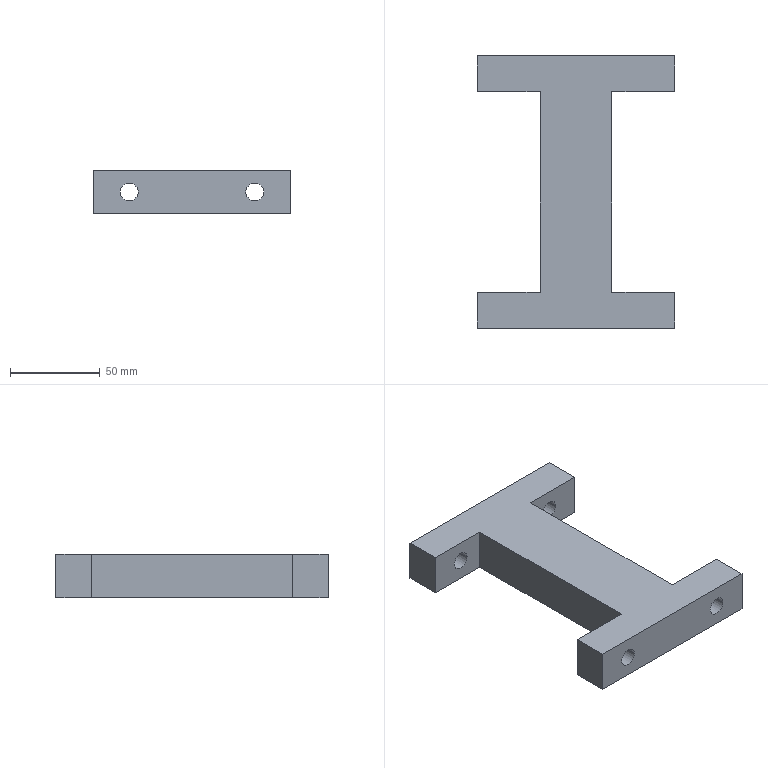Part | SolidWorks | features BaseBody 1 | 1 solid | 22 faces | box 110 x 152 x 24 mm | volume 206837 mm3 | plane 14 | cylinder 8 | commonest cylinder face diameters 10 x8
STEP:
#1=CARTESIAN_POINT('',(30.,-20.,0.));
#2=VERTEX_POINT('',#1);
#3=CARTESIAN_POINT('',(40.,-20.,0.));
#4=VERTEX_POINT('',#3);
#5=CARTESIAN_POINT('',(35.,-20.,0.));
#6=DIRECTION('',(0.,-1.,0.));
#7=DIRECTION('',(-1.,0.,0.));
#8=AXIS2_PLACEMENT_3D('',#5,#6,#7);
#9=CIRCLE('',#8,5.);
#10=EDGE_CURVE('',#2,#4,#9,.T.);
#11=ORIENTED_EDGE('',*,*,#10,.T.);
#12=CARTESIAN_POINT('',(40.,0.,0.));
#13=VERTEX_POINT('',#12);
#14=CARTESIAN_POINT('',(40.,-152.,0.));
#15=DIRECTION('',(0.,1.,0.));
#16=VECTOR('',#15,1000.);
#17=LINE('',#14,#16);
#18=EDGE_CURVE('',#4,#13,#17,.T.);
#19=ORIENTED_EDGE('',*,*,#18,.T.);
#20=CARTESIAN_POINT('',(30.,0.,0.));
#21=VERTEX_POINT('',#20);
#22=CARTESIAN_POINT('',(35.,0.,0.));
#23=DIRECTION('',(0.,1.,0.));
#24=DIRECTION('',(-1.,0.,0.));
#25=AXIS2_PLACEMENT_3D('',#22,#23,#24);
#26=CIRCLE('',#25,5.);
#27=EDGE_CURVE('',#13,#21,#26,.T.);
#28=ORIENTED_EDGE('',*,*,#27,.T.);
#29=CARTESIAN_POINT('',(30.,-152.,0.));
#30=DIRECTION('',(0.,1.,0.));
#31=VECTOR('',#30,1000.);
#32=LINE('',#29,#31);
#33=EDGE_CURVE('',#2,#21,#32,.T.);
#34=ORIENTED_EDGE('',*,*,#33,.F.);
#35=EDGE_LOOP('',(#11,#19,#28,#34));
#36=FACE_OUTER_BOUND('',#35,.T.);
#37=CARTESIAN_POINT('',(35.,-152.,0.));
#38=DIRECTION('',(0.,1.,0.));
#39=DIRECTION('',(-1.,0.,0.));
#40=AXIS2_PLACEMENT_3D('',#37,#38,#39);
#41=CYLINDRICAL_SURFACE('',#40,5.);
#42=ADVANCED_FACE('',(#36),#41,.F.);
#43=CARTESIAN_POINT('',(-40.,-20.,0.));
#44=VERTEX_POINT('',#43);
#45=CARTESIAN_POINT('',(-30.,-20.,0.));
#46=VERTEX_POINT('',#45);
#47=CARTESIAN_POINT('',(-35.,-20.,0.));
#48=DIRECTION('',(0.,-1.,0.));
#49=DIRECTION('',(-1.,0.,0.));
#50=AXIS2_PLACEMENT_3D('',#47,#48,#49);
#51=CIRCLE('',#50,5.);
#52=EDGE_CURVE('',#44,#46,#51,.T.);
#53=ORIENTED_EDGE('',*,*,#52,.T.);
#54=CARTESIAN_POINT('',(-30.,0.,0.));
#55=VERTEX_POINT('',#54);
#56=CARTESIAN_POINT('',(-30.,-152.,0.));
#57=DIRECTION('',(0.,1.,0.));
#58=VECTOR('',#57,1000.);
#59=LINE('',#56,#58);
#60=EDGE_CURVE('',#46,#55,#59,.T.);
#61=ORIENTED_EDGE('',*,*,#60,.T.);
#62=CARTESIAN_POINT('',(-40.,0.,0.));
#63=VERTEX_POINT('',#62);
#64=CARTESIAN_POINT('',(-35.,0.,0.));
#65=DIRECTION('',(0.,1.,0.));
#66=DIRECTION('',(-1.,0.,0.));
#67=AXIS2_PLACEMENT_3D('',#64,#65,#66);
#68=CIRCLE('',#67,5.);
#69=EDGE_CURVE('',#55,#63,#68,.T.);
#70=ORIENTED_EDGE('',*,*,#69,.T.);
#71=CARTESIAN_POINT('',(-40.,-152.,0.));
#72=DIRECTION('',(0.,1.,0.));
#73=VECTOR('',#72,1000.);
#74=LINE('',#71,#73);
#75=EDGE_CURVE('',#44,#63,#74,.T.);
#76=ORIENTED_EDGE('',*,*,#75,.F.);
#77=EDGE_LOOP('',(#53,#61,#70,#76));
#78=FACE_OUTER_BOUND('',#77,.T.);
#79=CARTESIAN_POINT('',(-35.,-152.,0.));
#80=DIRECTION('',(0.,1.,0.));
#81=DIRECTION('',(-1.,0.,0.));
#82=AXIS2_PLACEMENT_3D('',#79,#80,#81);
#83=CYLINDRICAL_SURFACE('',#82,5.);
#84=ADVANCED_FACE('',(#78),#83,.F.);
#85=CARTESIAN_POINT('',(30.,-152.,0.));
#86=VERTEX_POINT('',#85);
#87=CARTESIAN_POINT('',(40.,-152.,0.));
#88=VERTEX_POINT('',#87);
#89=CARTESIAN_POINT('',(35.,-152.,0.));
#90=DIRECTION('',(0.,-1.,0.));
#91=DIRECTION('',(-1.,0.,0.));
#92=AXIS2_PLACEMENT_3D('',#89,#90,#91);
#93=CIRCLE('',#92,5.);
#94=EDGE_CURVE('',#86,#88,#93,.T.);
#95=ORIENTED_EDGE('',*,*,#94,.T.);
#96=CARTESIAN_POINT('',(40.,-132.,0.));
#97=VERTEX_POINT('',#96);
#98=CARTESIAN_POINT('',(40.,-152.,0.));
#99=DIRECTION('',(0.,1.,0.));
#100=VECTOR('',#99,1000.);
#101=LINE('',#98,#100);
#102=EDGE_CURVE('',#88,#97,#101,.T.);
#103=ORIENTED_EDGE('',*,*,#102,.T.);
#104=CARTESIAN_POINT('',(30.,-132.,0.));
#105=VERTEX_POINT('',#104);
#106=CARTESIAN_POINT('',(35.,-132.,0.));
#107=DIRECTION('',(0.,1.,0.));
#108=DIRECTION('',(-1.,0.,0.));
#109=AXIS2_PLACEMENT_3D('',#106,#107,#108);
#110=CIRCLE('',#109,5.);
#111=EDGE_CURVE('',#97,#105,#110,.T.);
#112=ORIENTED_EDGE('',*,*,#111,.T.);
#113=CARTESIAN_POINT('',(30.,-152.,0.));
#114=DIRECTION('',(0.,1.,0.));
#115=VECTOR('',#114,1000.);
#116=LINE('',#113,#115);
#117=EDGE_CURVE('',#86,#105,#116,.T.);
#118=ORIENTED_EDGE('',*,*,#117,.F.);
#119=EDGE_LOOP('',(#95,#103,#112,#118));
#120=FACE_OUTER_BOUND('',#119,.T.);
#121=CARTESIAN_POINT('',(35.,-152.,0.));
#122=DIRECTION('',(0.,1.,0.));
#123=DIRECTION('',(-1.,0.,0.));
#124=AXIS2_PLACEMENT_3D('',#121,#122,#123);
#125=CYLINDRICAL_SURFACE('',#124,5.);
#126=ADVANCED_FACE('',(#120),#125,.F.);
#127=CARTESIAN_POINT('',(-40.,-152.,0.));
#128=VERTEX_POINT('',#127);
#129=CARTESIAN_POINT('',(-30.,-152.,0.));
#130=VERTEX_POINT('',#129);
#131=CARTESIAN_POINT('',(-35.,-152.,0.));
#132=DIRECTION('',(0.,-1.,0.));
#133=DIRECTION('',(-1.,0.,0.));
#134=AXIS2_PLACEMENT_3D('',#131,#132,#133);
#135=CIRCLE('',#134,5.);
#136=EDGE_CURVE('',#128,#130,#135,.T.);
#137=ORIENTED_EDGE('',*,*,#136,.T.);
#138=CARTESIAN_POINT('',(-30.,-132.,0.));
#139=VERTEX_POINT('',#138);
#140=CARTESIAN_POINT('',(-30.,-152.,0.));
#141=DIRECTION('',(0.,1.,0.));
#142=VECTOR('',#141,1000.);
#143=LINE('',#140,#142);
#144=EDGE_CURVE('',#130,#139,#143,.T.);
#145=ORIENTED_EDGE('',*,*,#144,.T.);
#146=CARTESIAN_POINT('',(-40.,-132.,0.));
#147=VERTEX_POINT('',#146);
#148=CARTESIAN_POINT('',(-35.,-132.,0.));
#149=DIRECTION('',(0.,1.,0.));
#150=DIRECTION('',(-1.,0.,0.));
#151=AXIS2_PLACEMENT_3D('',#148,#149,#150);
#152=CIRCLE('',#151,5.);
#153=EDGE_CURVE('',#139,#147,#152,.T.);
#154=ORIENTED_EDGE('',*,*,#153,.T.);
#155=CARTESIAN_POINT('',(-40.,-152.,0.));
#156=DIRECTION('',(0.,1.,0.));
#157=VECTOR('',#156,1000.);
#158=LINE('',#155,#157);
#159=EDGE_CURVE('',#128,#147,#158,.T.);
#160=ORIENTED_EDGE('',*,*,#159,.F.);
#161=EDGE_LOOP('',(#137,#145,#154,#160));
#162=FACE_OUTER_BOUND('',#161,.T.);
#163=CARTESIAN_POINT('',(-35.,-152.,0.));
#164=DIRECTION('',(0.,1.,0.));
#165=DIRECTION('',(-1.,0.,0.));
#166=AXIS2_PLACEMENT_3D('',#163,#164,#165);
#167=CYLINDRICAL_SURFACE('',#166,5.);
#168=ADVANCED_FACE('',(#162),#167,.F.);
#169=CARTESIAN_POINT('',(55.,-20.,12.));
#170=VERTEX_POINT('',#169);
#171=CARTESIAN_POINT('',(55.,0.,12.));
#172=VERTEX_POINT('',#171);
#173=CARTESIAN_POINT('',(55.,0.,12.));
#174=DIRECTION('',(0.,1.,0.));
#175=VECTOR('',#174,1000.);
#176=LINE('',#173,#175);
#177=EDGE_CURVE('',#170,#172,#176,.T.);
#178=ORIENTED_EDGE('',*,*,#177,.T.);
#179=CARTESIAN_POINT('',(-55.,0.,12.));
#180=VERTEX_POINT('',#179);
#181=CARTESIAN_POINT('',(0.,0.,12.));
#182=DIRECTION('',(-1.,0.,0.));
#183=VECTOR('',#182,1000.);
#184=LINE('',#181,#183);
#185=EDGE_CURVE('',#172,#180,#184,.T.);
#186=ORIENTED_EDGE('',*,*,#185,.T.);
#187=CARTESIAN_POINT('',(-55.,-20.,12.));
#188=VERTEX_POINT('',#187);
#189=CARTESIAN_POINT('',(-55.,0.,12.));
#190=DIRECTION('',(0.,-1.,0.));
#191=VECTOR('',#190,1000.);
#192=LINE('',#189,#191);
#193=EDGE_CURVE('',#180,#188,#192,.T.);
#194=ORIENTED_EDGE('',*,*,#193,.T.);
#195=CARTESIAN_POINT('',(-20.,-20.,12.));
#196=VERTEX_POINT('',#195);
#197=CARTESIAN_POINT('',(0.,-20.,12.));
#198=DIRECTION('',(1.,0.,0.));
#199=VECTOR('',#198,1000.);
#200=LINE('',#197,#199);
#201=EDGE_CURVE('',#188,#196,#200,.T.);
#202=ORIENTED_EDGE('',*,*,#201,.T.);
#203=CARTESIAN_POINT('',(-20.,-132.,12.));
#204=VERTEX_POINT('',#203);
#205=CARTESIAN_POINT('',(-20.,0.,12.));
#206=DIRECTION('',(0.,-1.,0.));
#207=VECTOR('',#206,1000.);
#208=LINE('',#205,#207);
#209=EDGE_CURVE('',#196,#204,#208,.T.);
#210=ORIENTED_EDGE('',*,*,#209,.T.);
#211=CARTESIAN_POINT('',(-55.,-132.,12.));
#212=VERTEX_POINT('',#211);
#213=CARTESIAN_POINT('',(0.,-132.,12.));
#214=DIRECTION('',(-1.,0.,0.));
#215=VECTOR('',#214,1000.);
#216=LINE('',#213,#215);
#217=EDGE_CURVE('',#204,#212,#216,.T.);
#218=ORIENTED_EDGE('',*,*,#217,.T.);
#219=CARTESIAN_POINT('',(-55.,-152.,12.));
#220=VERTEX_POINT('',#219);
#221=CARTESIAN_POINT('',(-55.,0.,12.));
#222=DIRECTION('',(0.,-1.,0.));
#223=VECTOR('',#222,1000.);
#224=LINE('',#221,#223);
#225=EDGE_CURVE('',#212,#220,#224,.T.);
#226=ORIENTED_EDGE('',*,*,#225,.T.);
#227=CARTESIAN_POINT('',(55.,-152.,12.));
#228=VERTEX_POINT('',#227);
#229=CARTESIAN_POINT('',(0.,-152.,12.));
#230=DIRECTION('',(1.,0.,0.));
#231=VECTOR('',#230,1000.);
#232=LINE('',#229,#231);
#233=EDGE_CURVE('',#220,#228,#232,.T.);
#234=ORIENTED_EDGE('',*,*,#233,.T.);
#235=CARTESIAN_POINT('',(55.,-132.,12.));
#236=VERTEX_POINT('',#235);
#237=CARTESIAN_POINT('',(55.,0.,12.));
#238=DIRECTION('',(0.,1.,0.));
#239=VECTOR('',#238,1000.);
#240=LINE('',#237,#239);
#241=EDGE_CURVE('',#228,#236,#240,.T.);
#242=ORIENTED_EDGE('',*,*,#241,.T.);
#243=CARTESIAN_POINT('',(20.,-132.,12.));
#244=VERTEX_POINT('',#243);
#245=CARTESIAN_POINT('',(0.,-132.,12.));
#246=DIRECTION('',(-1.,0.,0.));
#247=VECTOR('',#246,1000.);
#248=LINE('',#245,#247);
#249=EDGE_CURVE('',#236,#244,#248,.T.);
#250=ORIENTED_EDGE('',*,*,#249,.T.);
#251=CARTESIAN_POINT('',(20.,-20.,12.));
#252=VERTEX_POINT('',#251);
#253=CARTESIAN_POINT('',(20.,0.,12.));
#254=DIRECTION('',(0.,1.,0.));
#255=VECTOR('',#254,1000.);
#256=LINE('',#253,#255);
#257=EDGE_CURVE('',#244,#252,#256,.T.);
#258=ORIENTED_EDGE('',*,*,#257,.T.);
#259=CARTESIAN_POINT('',(0.,-20.,12.));
#260=DIRECTION('',(1.,0.,0.));
#261=VECTOR('',#260,1000.);
#262=LINE('',#259,#261);
#263=EDGE_CURVE('',#252,#170,#262,.T.);
#264=ORIENTED_EDGE('',*,*,#263,.T.);
#265=EDGE_LOOP('',(#178,#186,#194,#202,#210,#218,#226,#234,#242,#250,#258,#264));
#266=FACE_OUTER_BOUND('',#265,.T.);
#267=CARTESIAN_POINT('',(0.,0.,12.));
#268=DIRECTION('',(0.,0.,1.));
#269=DIRECTION('',(1.,0.,0.));
#270=AXIS2_PLACEMENT_3D('',#267,#268,#269);
#271=PLANE('',#270);
#272=ADVANCED_FACE('',(#266),#271,.T.);
#273=CARTESIAN_POINT('',(-55.,0.,-12.));
#274=VERTEX_POINT('',#273);
#275=CARTESIAN_POINT('',(-55.,0.,12.));
#276=DIRECTION('',(0.,0.,-1.));
#277=VECTOR('',#276,1000.);
#278=LINE('',#275,#277);
#279=EDGE_CURVE('',#180,#274,#278,.T.);
#280=ORIENTED_EDGE('',*,*,#279,.F.);
#281=ORIENTED_EDGE('',*,*,#185,.F.);
#282=CARTESIAN_POINT('',(55.,0.,-12.));
#283=VERTEX_POINT('',#282);
#284=CARTESIAN_POINT('',(55.,0.,12.));
#285=DIRECTION('',(0.,0.,1.));
#286=VECTOR('',#285,1000.);
#287=LINE('',#284,#286);
#288=EDGE_CURVE('',#283,#172,#287,.T.);
#289=ORIENTED_EDGE('',*,*,#288,.F.);
#290=CARTESIAN_POINT('',(-55.,0.,-12.));
#291=DIRECTION('',(1.,0.,0.));
#292=VECTOR('',#291,1000.);
#293=LINE('',#290,#292);
#294=EDGE_CURVE('',#274,#283,#293,.T.);
#295=ORIENTED_EDGE('',*,*,#294,.F.);
#296=EDGE_LOOP('',(#280,#281,#289,#295));
#297=FACE_OUTER_BOUND('',#296,.T.);
#298=CARTESIAN_POINT('',(35.,0.,0.));
#299=DIRECTION('',(0.,1.,0.));
#300=DIRECTION('',(-1.,0.,0.));
#301=AXIS2_PLACEMENT_3D('',#298,#299,#300);
#302=CIRCLE('',#301,5.);
#303=EDGE_CURVE('',#21,#13,#302,.T.);
#304=ORIENTED_EDGE('',*,*,#303,.F.);
#305=ORIENTED_EDGE('',*,*,#27,.F.);
#306=EDGE_LOOP('',(#304,#305));
#307=FACE_BOUND('',#306,.T.);
#308=CARTESIAN_POINT('',(-35.,0.,0.));
#309=DIRECTION('',(0.,1.,0.));
#310=DIRECTION('',(-1.,0.,0.));
#311=AXIS2_PLACEMENT_3D('',#308,#309,#310);
#312=CIRCLE('',#311,5.);
#313=EDGE_CURVE('',#63,#55,#312,.T.);
#314=ORIENTED_EDGE('',*,*,#313,.F.);
#315=ORIENTED_EDGE('',*,*,#69,.F.);
#316=EDGE_LOOP('',(#314,#315));
#317=FACE_BOUND('',#316,.T.);
#318=CARTESIAN_POINT('',(-55.,0.,12.));
#319=DIRECTION('',(0.,-1.,0.));
#320=DIRECTION('',(1.,0.,0.));
#321=AXIS2_PLACEMENT_3D('',#318,#319,#320);
#322=PLANE('',#321);
#323=ADVANCED_FACE('',(#297,#307,#317),#322,.F.);
#324=ORIENTED_EDGE('',*,*,#288,.T.);
#325=ORIENTED_EDGE('',*,*,#177,.F.);
#326=CARTESIAN_POINT('',(55.,-20.,-12.));
#327=VERTEX_POINT('',#326);
#328=CARTESIAN_POINT('',(55.,-20.,12.));
#329=DIRECTION('',(0.,0.,1.));
#330=VECTOR('',#329,1000.);
#331=LINE('',#328,#330);
#332=EDGE_CURVE('',#327,#170,#331,.T.);
#333=ORIENTED_EDGE('',*,*,#332,.F.);
#334=CARTESIAN_POINT('',(55.,0.,-12.));
#335=DIRECTION('',(0.,-1.,0.));
#336=VECTOR('',#335,1000.);
#337=LINE('',#334,#336);
#338=EDGE_CURVE('',#283,#327,#337,.T.);
#339=ORIENTED_EDGE('',*,*,#338,.F.);
#340=EDGE_LOOP('',(#324,#325,#333,#339));
#341=FACE_OUTER_BOUND('',#340,.T.);
#342=CARTESIAN_POINT('',(55.,0.,12.));
#343=DIRECTION('',(-1.,0.,0.));
#344=DIRECTION('',(0.,0.,1.));
#345=AXIS2_PLACEMENT_3D('',#342,#343,#344);
#346=PLANE('',#345);
#347=ADVANCED_FACE('',(#341),#346,.F.);
#348=ORIENTED_EDGE('',*,*,#332,.T.);
#349=ORIENTED_EDGE('',*,*,#263,.F.);
#350=CARTESIAN_POINT('',(20.,-20.,-12.));
#351=VERTEX_POINT('',#350);
#352=CARTESIAN_POINT('',(20.,-20.,12.));
#353=DIRECTION('',(0.,0.,1.));
#354=VECTOR('',#353,1000.);
#355=LINE('',#352,#354);
#356=EDGE_CURVE('',#351,#252,#355,.T.);
#357=ORIENTED_EDGE('',*,*,#356,.F.);
#358=CARTESIAN_POINT('',(55.,-20.,-12.));
#359=DIRECTION('',(-1.,0.,0.));
#360=VECTOR('',#359,1000.);
#361=LINE('',#358,#360);
#362=EDGE_CURVE('',#327,#351,#361,.T.);
#363=ORIENTED_EDGE('',*,*,#362,.F.);
#364=EDGE_LOOP('',(#348,#349,#357,#363));
#365=FACE_OUTER_BOUND('',#364,.T.);
#366=ORIENTED_EDGE('',*,*,#10,.F.);
#367=CARTESIAN_POINT('',(35.,-20.,0.));
#368=DIRECTION('',(0.,-1.,0.));
#369=DIRECTION('',(-1.,0.,0.));
#370=AXIS2_PLACEMENT_3D('',#367,#368,#369);
#371=CIRCLE('',#370,5.);
#372=EDGE_CURVE('',#4,#2,#371,.T.);
#373=ORIENTED_EDGE('',*,*,#372,.F.);
#374=EDGE_LOOP('',(#366,#373));
#375=FACE_BOUND('',#374,.T.);
#376=CARTESIAN_POINT('',(55.,-20.,12.));
#377=DIRECTION('',(0.,1.,0.));
#378=DIRECTION('',(0.,0.,1.));
#379=AXIS2_PLACEMENT_3D('',#376,#377,#378);
#380=PLANE('',#379);
#381=ADVANCED_FACE('',(#365,#375),#380,.F.);
#382=ORIENTED_EDGE('',*,*,#356,.T.);
#383=ORIENTED_EDGE('',*,*,#257,.F.);
#384=CARTESIAN_POINT('',(20.,-132.,-12.));
#385=VERTEX_POINT('',#384);
#386=CARTESIAN_POINT('',(20.,-132.,12.));
#387=DIRECTION('',(0.,0.,1.));
#388=VECTOR('',#387,1000.);
#389=LINE('',#386,#388);
#390=EDGE_CURVE('',#385,#244,#389,.T.);
#391=ORIENTED_EDGE('',*,*,#390,.F.);
#392=CARTESIAN_POINT('',(20.,-20.,-12.));
#393=DIRECTION('',(0.,-1.,0.));
#394=VECTOR('',#393,1000.);
#395=LINE('',#392,#394);
#396=EDGE_CURVE('',#351,#385,#395,.T.);
#397=ORIENTED_EDGE('',*,*,#396,.F.);
#398=EDGE_LOOP('',(#382,#383,#391,#397));
#399=FACE_OUTER_BOUND('',#398,.T.);
#400=CARTESIAN_POINT('',(20.,-20.,12.));
#401=DIRECTION('',(-1.,0.,0.));
#402=DIRECTION('',(0.,-1.,0.));
#403=AXIS2_PLACEMENT_3D('',#400,#401,#402);
#404=PLANE('',#403);
#405=ADVANCED_FACE('',(#399),#404,.F.);
#406=ORIENTED_EDGE('',*,*,#390,.T.);
#407=ORIENTED_EDGE('',*,*,#249,.F.);
#408=CARTESIAN_POINT('',(55.,-132.,-12.));
#409=VERTEX_POINT('',#408);
#410=CARTESIAN_POINT('',(55.,-132.,12.));
#411=DIRECTION('',(0.,0.,1.));
#412=VECTOR('',#411,1000.);
#413=LINE('',#410,#412);
#414=EDGE_CURVE('',#409,#236,#413,.T.);
#415=ORIENTED_EDGE('',*,*,#414,.F.);
#416=CARTESIAN_POINT('',(20.,-132.,-12.));
#417=DIRECTION('',(1.,0.,0.));
#418=VECTOR('',#417,1000.);
#419=LINE('',#416,#418);
#420=EDGE_CURVE('',#385,#409,#419,.T.);
#421=ORIENTED_EDGE('',*,*,#420,.F.);
#422=EDGE_LOOP('',(#406,#407,#415,#421));
#423=FACE_OUTER_BOUND('',#422,.T.);
#424=CARTESIAN_POINT('',(35.,-132.,0.));
#425=DIRECTION('',(0.,1.,0.));
#426=DIRECTION('',(-1.,0.,0.));
#427=AXIS2_PLACEMENT_3D('',#424,#425,#426);
#428=CIRCLE('',#427,5.);
#429=EDGE_CURVE('',#105,#97,#428,.T.);
#430=ORIENTED_EDGE('',*,*,#429,.F.);
#431=ORIENTED_EDGE('',*,*,#111,.F.);
#432=EDGE_LOOP('',(#430,#431));
#433=FACE_BOUND('',#432,.T.);
#434=CARTESIAN_POINT('',(20.,-132.,12.));
#435=DIRECTION('',(0.,-1.,0.));
#436=DIRECTION('',(0.,0.,-1.));
#437=AXIS2_PLACEMENT_3D('',#434,#435,#436);
#438=PLANE('',#437);
#439=ADVANCED_FACE('',(#423,#433),#438,.F.);
#440=ORIENTED_EDGE('',*,*,#414,.T.);
#441=ORIENTED_EDGE('',*,*,#241,.F.);
#442=CARTESIAN_POINT('',(55.,-152.,-12.));
#443=VERTEX_POINT('',#442);
#444=CARTESIAN_POINT('',(55.,-152.,12.));
#445=DIRECTION('',(0.,0.,1.));
#446=VECTOR('',#445,1000.);
#447=LINE('',#444,#446);
#448=EDGE_CURVE('',#443,#228,#447,.T.);
#449=ORIENTED_EDGE('',*,*,#448,.F.);
#450=CARTESIAN_POINT('',(55.,-132.,-12.));
#451=DIRECTION('',(0.,-1.,0.));
#452=VECTOR('',#451,1000.);
#453=LINE('',#450,#452);
#454=EDGE_CURVE('',#409,#443,#453,.T.);
#455=ORIENTED_EDGE('',*,*,#454,.F.);
#456=EDGE_LOOP('',(#440,#441,#449,#455));
#457=FACE_OUTER_BOUND('',#456,.T.);
#458=CARTESIAN_POINT('',(55.,-132.,12.));
#459=DIRECTION('',(-1.,0.,0.));
#460=DIRECTION('',(0.,0.,1.));
#461=AXIS2_PLACEMENT_3D('',#458,#459,#460);
#462=PLANE('',#461);
#463=ADVANCED_FACE('',(#457),#462,.F.);
#464=ORIENTED_EDGE('',*,*,#448,.T.);
#465=ORIENTED_EDGE('',*,*,#233,.F.);
#466=CARTESIAN_POINT('',(-55.,-152.,-12.));
#467=VERTEX_POINT('',#466);
#468=CARTESIAN_POINT('',(-55.,-152.,12.));
#469=DIRECTION('',(0.,0.,1.));
#470=VECTOR('',#469,1000.);
#471=LINE('',#468,#470);
#472=EDGE_CURVE('',#467,#220,#471,.T.);
#473=ORIENTED_EDGE('',*,*,#472,.F.);
#474=CARTESIAN_POINT('',(-55.,-152.,-12.));
#475=DIRECTION('',(-1.,0.,0.));
#476=VECTOR('',#475,1000.);
#477=LINE('',#474,#476);
#478=EDGE_CURVE('',#443,#467,#477,.T.);
#479=ORIENTED_EDGE('',*,*,#478,.F.);
#480=EDGE_LOOP('',(#464,#465,#473,#479));
#481=FACE_OUTER_BOUND('',#480,.T.);
#482=ORIENTED_EDGE('',*,*,#94,.F.);
#483=CARTESIAN_POINT('',(35.,-152.,0.));
#484=DIRECTION('',(0.,-1.,0.));
#485=DIRECTION('',(-1.,0.,0.));
#486=AXIS2_PLACEMENT_3D('',#483,#484,#485);
#487=CIRCLE('',#486,5.);
#488=EDGE_CURVE('',#88,#86,#487,.T.);
#489=ORIENTED_EDGE('',*,*,#488,.F.);
#490=EDGE_LOOP('',(#482,#489));
#491=FACE_BOUND('',#490,.T.);
#492=ORIENTED_EDGE('',*,*,#136,.F.);
#493=CARTESIAN_POINT('',(-35.,-152.,0.));
#494=DIRECTION('',(0.,-1.,0.));
#495=DIRECTION('',(-1.,0.,0.));
#496=AXIS2_PLACEMENT_3D('',#493,#494,#495);
#497=CIRCLE('',#496,5.);
#498=EDGE_CURVE('',#130,#128,#497,.T.);
#499=ORIENTED_EDGE('',*,*,#498,.F.);
#500=EDGE_LOOP('',(#492,#499));
#501=FACE_BOUND('',#500,.T.);
#502=CARTESIAN_POINT('',(-55.,-152.,12.));
#503=DIRECTION('',(0.,1.,0.));
#504=DIRECTION('',(0.,0.,1.));
#505=AXIS2_PLACEMENT_3D('',#502,#503,#504);
#506=PLANE('',#505);
#507=ADVANCED_FACE('',(#481,#491,#501),#506,.F.);
#508=ORIENTED_EDGE('',*,*,#472,.T.);
#509=ORIENTED_EDGE('',*,*,#225,.F.);
#510=CARTESIAN_POINT('',(-55.,-132.,-12.));
#511=VERTEX_POINT('',#510);
#512=CARTESIAN_POINT('',(-55.,-132.,12.));
#513=DIRECTION('',(0.,0.,1.));
#514=VECTOR('',#513,1000.);
#515=LINE('',#512,#514);
#516=EDGE_CURVE('',#511,#212,#515,.T.);
#517=ORIENTED_EDGE('',*,*,#516,.F.);
#518=CARTESIAN_POINT('',(-55.,-132.,-12.));
#519=DIRECTION('',(0.,1.,0.));
#520=VECTOR('',#519,1000.);
#521=LINE('',#518,#520);
#522=EDGE_CURVE('',#467,#511,#521,.T.);
#523=ORIENTED_EDGE('',*,*,#522,.F.);
#524=EDGE_LOOP('',(#508,#509,#517,#523));
#525=FACE_OUTER_BOUND('',#524,.T.);
#526=CARTESIAN_POINT('',(-55.,-132.,12.));
#527=DIRECTION('',(1.,0.,0.));
#528=DIRECTION('',(0.,0.,-1.));
#529=AXIS2_PLACEMENT_3D('',#526,#527,#528);
#530=PLANE('',#529);
#531=ADVANCED_FACE('',(#525),#530,.F.);
#532=ORIENTED_EDGE('',*,*,#516,.T.);
#533=ORIENTED_EDGE('',*,*,#217,.F.);
#534=CARTESIAN_POINT('',(-20.,-132.,-12.));
#535=VERTEX_POINT('',#534);
#536=CARTESIAN_POINT('',(-20.,-132.,12.));
#537=DIRECTION('',(0.,0.,1.));
#538=VECTOR('',#537,1000.);
#539=LINE('',#536,#538);
#540=EDGE_CURVE('',#535,#204,#539,.T.);
#541=ORIENTED_EDGE('',*,*,#540,.F.);
#542=CARTESIAN_POINT('',(-20.,-132.,-12.));
#543=DIRECTION('',(1.,0.,0.));
#544=VECTOR('',#543,1000.);
#545=LINE('',#542,#544);
#546=EDGE_CURVE('',#511,#535,#545,.T.);
#547=ORIENTED_EDGE('',*,*,#546,.F.);
#548=EDGE_LOOP('',(#532,#533,#541,#547));
#549=FACE_OUTER_BOUND('',#548,.T.);
#550=CARTESIAN_POINT('',(-35.,-132.,0.));
#551=DIRECTION('',(0.,1.,0.));
#552=DIRECTION('',(-1.,0.,0.));
#553=AXIS2_PLACEMENT_3D('',#550,#551,#552);
#554=CIRCLE('',#553,5.);
#555=EDGE_CURVE('',#147,#139,#554,.T.);
#556=ORIENTED_EDGE('',*,*,#555,.F.);
#557=ORIENTED_EDGE('',*,*,#153,.F.);
#558=EDGE_LOOP('',(#556,#557));
#559=FACE_BOUND('',#558,.T.);
#560=CARTESIAN_POINT('',(-20.,-132.,12.));
#561=DIRECTION('',(0.,-1.,0.));
#562=DIRECTION('',(0.,0.,-1.));
#563=AXIS2_PLACEMENT_3D('',#560,#561,#562);
#564=PLANE('',#563);
#565=ADVANCED_FACE('',(#549,#559),#564,.F.);
#566=ORIENTED_EDGE('',*,*,#540,.T.);
#567=ORIENTED_EDGE('',*,*,#209,.F.);
#568=CARTESIAN_POINT('',(-20.,-20.,-12.));
#569=VERTEX_POINT('',#568);
#570=CARTESIAN_POINT('',(-20.,-20.,12.));
#571=DIRECTION('',(0.,0.,1.));
#572=VECTOR('',#571,1000.);
#573=LINE('',#570,#572);
#574=EDGE_CURVE('',#569,#196,#573,.T.);
#575=ORIENTED_EDGE('',*,*,#574,.F.);
#576=CARTESIAN_POINT('',(-20.,-20.,-12.));
#577=DIRECTION('',(0.,1.,0.));
#578=VECTOR('',#577,1000.);
#579=LINE('',#576,#578);
#580=EDGE_CURVE('',#535,#569,#579,.T.);
#581=ORIENTED_EDGE('',*,*,#580,.F.);
#582=EDGE_LOOP('',(#566,#567,#575,#581));
#583=FACE_OUTER_BOUND('',#582,.T.);
#584=CARTESIAN_POINT('',(-20.,-20.,12.));
#585=DIRECTION('',(1.,0.,0.));
#586=DIRECTION('',(0.,1.,0.));
#587=AXIS2_PLACEMENT_3D('',#584,#585,#586);
#588=PLANE('',#587);
#589=ADVANCED_FACE('',(#583),#588,.F.);
#590=ORIENTED_EDGE('',*,*,#574,.T.);
#591=ORIENTED_EDGE('',*,*,#201,.F.);
#592=CARTESIAN_POINT('',(-55.,-20.,-12.));
#593=VERTEX_POINT('',#592);
#594=CARTESIAN_POINT('',(-55.,-20.,12.));
#595=DIRECTION('',(0.,0.,1.));
#596=VECTOR('',#595,1000.);
#597=LINE('',#594,#596);
#598=EDGE_CURVE('',#593,#188,#597,.T.);
#599=ORIENTED_EDGE('',*,*,#598,.F.);
#600=CARTESIAN_POINT('',(-55.,-20.,-12.));
#601=DIRECTION('',(-1.,0.,0.));
#602=VECTOR('',#601,1000.);
#603=LINE('',#600,#602);
#604=EDGE_CURVE('',#569,#593,#603,.T.);
#605=ORIENTED_EDGE('',*,*,#604,.F.);
#606=EDGE_LOOP('',(#590,#591,#599,#605));
#607=FACE_OUTER_BOUND('',#606,.T.);
#608=ORIENTED_EDGE('',*,*,#52,.F.);
#609=CARTESIAN_POINT('',(-35.,-20.,0.));
#610=DIRECTION('',(0.,-1.,0.));
#611=DIRECTION('',(-1.,0.,0.));
#612=AXIS2_PLACEMENT_3D('',#609,#610,#611);
#613=CIRCLE('',#612,5.);
#614=EDGE_CURVE('',#46,#44,#613,.T.);
#615=ORIENTED_EDGE('',*,*,#614,.F.);
#616=EDGE_LOOP('',(#608,#615));
#617=FACE_BOUND('',#616,.T.);
#618=CARTESIAN_POINT('',(-55.,-20.,12.));
#619=DIRECTION('',(0.,1.,0.));
#620=DIRECTION('',(0.,0.,1.));
#621=AXIS2_PLACEMENT_3D('',#618,#619,#620);
#622=PLANE('',#621);
#623=ADVANCED_FACE('',(#607,#617),#622,.F.);
#624=ORIENTED_EDGE('',*,*,#598,.T.);
#625=ORIENTED_EDGE('',*,*,#193,.F.);
#626=ORIENTED_EDGE('',*,*,#279,.T.);
#627=CARTESIAN_POINT('',(-55.,0.,-12.));
#628=DIRECTION('',(0.,1.,0.));
#629=VECTOR('',#628,1000.);
#630=LINE('',#627,#629);
#631=EDGE_CURVE('',#593,#274,#630,.T.);
#632=ORIENTED_EDGE('',*,*,#631,.F.);
#633=EDGE_LOOP('',(#624,#625,#626,#632));
#634=FACE_OUTER_BOUND('',#633,.T.);
#635=CARTESIAN_POINT('',(-55.,0.,12.));
#636=DIRECTION('',(1.,0.,0.));
#637=DIRECTION('',(0.,0.,-1.));
#638=AXIS2_PLACEMENT_3D('',#635,#636,#637);
#639=PLANE('',#638);
#640=ADVANCED_FACE('',(#634),#639,.F.);
#641=ORIENTED_EDGE('',*,*,#294,.T.);
#642=ORIENTED_EDGE('',*,*,#338,.T.);
#643=ORIENTED_EDGE('',*,*,#362,.T.);
#644=ORIENTED_EDGE('',*,*,#396,.T.);
#645=ORIENTED_EDGE('',*,*,#420,.T.);
#646=ORIENTED_EDGE('',*,*,#454,.T.);
#647=ORIENTED_EDGE('',*,*,#478,.T.);
#648=ORIENTED_EDGE('',*,*,#522,.T.);
#649=ORIENTED_EDGE('',*,*,#546,.T.);
#650=ORIENTED_EDGE('',*,*,#580,.T.);
#651=ORIENTED_EDGE('',*,*,#604,.T.);
#652=ORIENTED_EDGE('',*,*,#631,.T.);
#653=EDGE_LOOP('',(#641,#642,#643,#644,#645,#646,#647,#648,#649,#650,#651,#652));
#654=FACE_OUTER_BOUND('',#653,.T.);
#655=CARTESIAN_POINT('',(0.,0.,-12.));
#656=DIRECTION('',(0.,0.,1.));
#657=DIRECTION('',(1.,0.,0.));
#658=AXIS2_PLACEMENT_3D('',#655,#656,#657);
#659=PLANE('',#658);
#660=ADVANCED_FACE('',(#654),#659,.F.);
#661=ORIENTED_EDGE('',*,*,#18,.F.);
#662=ORIENTED_EDGE('',*,*,#372,.T.);
#663=ORIENTED_EDGE('',*,*,#33,.T.);
#664=ORIENTED_EDGE('',*,*,#303,.T.);
#665=EDGE_LOOP('',(#661,#662,#663,#664));
#666=FACE_OUTER_BOUND('',#665,.T.);
#667=CARTESIAN_POINT('',(35.,-152.,0.));
#668=DIRECTION('',(0.,1.,0.));
#669=DIRECTION('',(-1.,0.,0.));
#670=AXIS2_PLACEMENT_3D('',#667,#668,#669);
#671=CYLINDRICAL_SURFACE('',#670,5.);
#672=ADVANCED_FACE('',(#666),#671,.F.);
#673=ORIENTED_EDGE('',*,*,#60,.F.);
#674=ORIENTED_EDGE('',*,*,#614,.T.);
#675=ORIENTED_EDGE('',*,*,#75,.T.);
#676=ORIENTED_EDGE('',*,*,#313,.T.);
#677=EDGE_LOOP('',(#673,#674,#675,#676));
#678=FACE_OUTER_BOUND('',#677,.T.);
#679=CARTESIAN_POINT('',(-35.,-152.,0.));
#680=DIRECTION('',(0.,1.,0.));
#681=DIRECTION('',(-1.,0.,0.));
#682=AXIS2_PLACEMENT_3D('',#679,#680,#681);
#683=CYLINDRICAL_SURFACE('',#682,5.);
#684=ADVANCED_FACE('',(#678),#683,.F.);
#685=ORIENTED_EDGE('',*,*,#102,.F.);
#686=ORIENTED_EDGE('',*,*,#488,.T.);
#687=ORIENTED_EDGE('',*,*,#117,.T.);
#688=ORIENTED_EDGE('',*,*,#429,.T.);
#689=EDGE_LOOP('',(#685,#686,#687,#688));
#690=FACE_OUTER_BOUND('',#689,.T.);
#691=CARTESIAN_POINT('',(35.,-152.,0.));
#692=DIRECTION('',(0.,1.,0.));
#693=DIRECTION('',(-1.,0.,0.));
#694=AXIS2_PLACEMENT_3D('',#691,#692,#693);
#695=CYLINDRICAL_SURFACE('',#694,5.);
#696=ADVANCED_FACE('',(#690),#695,.F.);
#697=ORIENTED_EDGE('',*,*,#144,.F.);
#698=ORIENTED_EDGE('',*,*,#498,.T.);
#699=ORIENTED_EDGE('',*,*,#159,.T.);
#700=ORIENTED_EDGE('',*,*,#555,.T.);
#701=EDGE_LOOP('',(#697,#698,#699,#700));
#702=FACE_OUTER_BOUND('',#701,.T.);
#703=CARTESIAN_POINT('',(-35.,-152.,0.));
#704=DIRECTION('',(0.,1.,0.));
#705=DIRECTION('',(-1.,0.,0.));
#706=AXIS2_PLACEMENT_3D('',#703,#704,#705);
#707=CYLINDRICAL_SURFACE('',#706,5.);
#708=ADVANCED_FACE('',(#702),#707,.F.);
#709=CLOSED_SHELL('',(#42,#84,#126,#168,#272,#323,#347,#381,#405,#439,#463,#507,#531,#565,#589,#623,#640,#660,#672,#684,#696,#708));
#710=MANIFOLD_SOLID_BREP('',#709);
#711=CARTESIAN_POINT('',(0.,0.,0.));
#712=DIRECTION('',(0.,0.,1.));
#713=DIRECTION('',(1.,0.,0.));
#714=AXIS2_PLACEMENT_3D('',#711,#712,#713);
#715=(LENGTH_UNIT()NAMED_UNIT(*)SI_UNIT(.MILLI.,.METRE.));
#716=UNCERTAINTY_MEASURE_WITH_UNIT(LENGTH_MEASURE(0.00001),#715,'','');
#717=(NAMED_UNIT(*)PLANE_ANGLE_UNIT()SI_UNIT($,.RADIAN.));
#718=(NAMED_UNIT(*)SI_UNIT($,.STERADIAN.)SOLID_ANGLE_UNIT());
#719=(GEOMETRIC_REPRESENTATION_CONTEXT(3)GLOBAL_UNCERTAINTY_ASSIGNED_CONTEXT((#716))GLOBAL_UNIT_ASSIGNED_CONTEXT((#715,#717,#718))REPRESENTATION_CONTEXT('',''));
#720=ADVANCED_BREP_SHAPE_REPRESENTATION('',(#710,#714),#719);